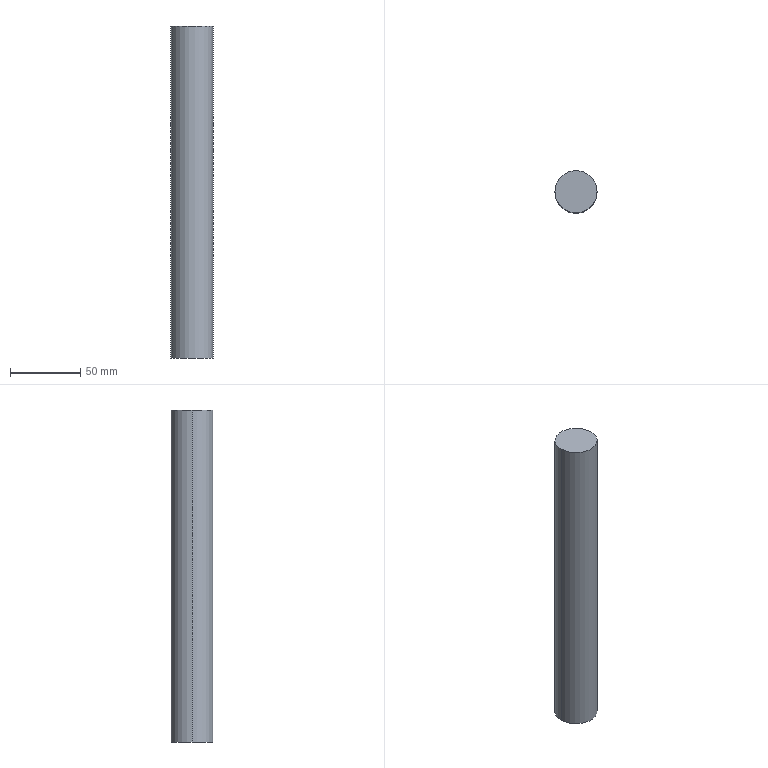Part | SolidWorks | features Extrusion 1 | 1 solid | 4 faces | box 30 x 30 x 236 mm | volume 166819 mm3 | cylinder 2 | plane 2 | commonest cylinder face diameters 30 x2
STEP:
#1=CARTESIAN_POINT('',(15.,0.,236.));
#2=VERTEX_POINT('',#1);
#3=CARTESIAN_POINT('',(-15.,0.,236.));
#4=VERTEX_POINT('',#3);
#5=CARTESIAN_POINT('',(0.,0.,236.));
#6=DIRECTION('',(0.,0.,1.));
#7=DIRECTION('',(1.,0.,0.));
#8=AXIS2_PLACEMENT_3D('',#5,#6,#7);
#9=CIRCLE('',#8,15.);
#10=EDGE_CURVE('',#2,#4,#9,.T.);
#11=ORIENTED_EDGE('',*,*,#10,.F.);
#12=CARTESIAN_POINT('',(15.,0.,0.));
#13=VERTEX_POINT('',#12);
#14=CARTESIAN_POINT('',(15.,0.,236.));
#15=DIRECTION('',(0.,0.,-1.));
#16=VECTOR('',#15,1000.);
#17=LINE('',#14,#16);
#18=EDGE_CURVE('',#2,#13,#17,.T.);
#19=ORIENTED_EDGE('',*,*,#18,.T.);
#20=CARTESIAN_POINT('',(-15.,0.,0.));
#21=VERTEX_POINT('',#20);
#22=CARTESIAN_POINT('',(0.,0.,0.));
#23=DIRECTION('',(0.,0.,1.));
#24=DIRECTION('',(1.,0.,0.));
#25=AXIS2_PLACEMENT_3D('',#22,#23,#24);
#26=CIRCLE('',#25,15.);
#27=EDGE_CURVE('',#13,#21,#26,.T.);
#28=ORIENTED_EDGE('',*,*,#27,.T.);
#29=CARTESIAN_POINT('',(-15.,0.,236.));
#30=DIRECTION('',(0.,0.,-1.));
#31=VECTOR('',#30,1000.);
#32=LINE('',#29,#31);
#33=EDGE_CURVE('',#4,#21,#32,.T.);
#34=ORIENTED_EDGE('',*,*,#33,.F.);
#35=EDGE_LOOP('',(#11,#19,#28,#34));
#36=FACE_OUTER_BOUND('',#35,.T.);
#37=CARTESIAN_POINT('',(0.,0.,236.));
#38=DIRECTION('',(0.,0.,-1.));
#39=DIRECTION('',(-1.,0.,0.));
#40=AXIS2_PLACEMENT_3D('',#37,#38,#39);
#41=CYLINDRICAL_SURFACE('',#40,15.);
#42=ADVANCED_FACE('',(#36),#41,.T.);
#43=ORIENTED_EDGE('',*,*,#18,.F.);
#44=CARTESIAN_POINT('',(0.,0.,236.));
#45=DIRECTION('',(0.,0.,1.));
#46=DIRECTION('',(1.,0.,0.));
#47=AXIS2_PLACEMENT_3D('',#44,#45,#46);
#48=CIRCLE('',#47,15.);
#49=EDGE_CURVE('',#4,#2,#48,.T.);
#50=ORIENTED_EDGE('',*,*,#49,.F.);
#51=ORIENTED_EDGE('',*,*,#33,.T.);
#52=CARTESIAN_POINT('',(0.,0.,0.));
#53=DIRECTION('',(0.,0.,1.));
#54=DIRECTION('',(1.,0.,0.));
#55=AXIS2_PLACEMENT_3D('',#52,#53,#54);
#56=CIRCLE('',#55,15.);
#57=EDGE_CURVE('',#21,#13,#56,.T.);
#58=ORIENTED_EDGE('',*,*,#57,.T.);
#59=EDGE_LOOP('',(#43,#50,#51,#58));
#60=FACE_OUTER_BOUND('',#59,.T.);
#61=CARTESIAN_POINT('',(0.,0.,236.));
#62=DIRECTION('',(0.,0.,-1.));
#63=DIRECTION('',(-1.,0.,0.));
#64=AXIS2_PLACEMENT_3D('',#61,#62,#63);
#65=CYLINDRICAL_SURFACE('',#64,15.);
#66=ADVANCED_FACE('',(#60),#65,.T.);
#67=ORIENTED_EDGE('',*,*,#49,.T.);
#68=ORIENTED_EDGE('',*,*,#10,.T.);
#69=EDGE_LOOP('',(#67,#68));
#70=FACE_OUTER_BOUND('',#69,.T.);
#71=CARTESIAN_POINT('',(0.,0.,236.));
#72=DIRECTION('',(0.,0.,1.));
#73=DIRECTION('',(1.,0.,0.));
#74=AXIS2_PLACEMENT_3D('',#71,#72,#73);
#75=PLANE('',#74);
#76=ADVANCED_FACE('',(#70),#75,.T.);
#77=ORIENTED_EDGE('',*,*,#57,.F.);
#78=ORIENTED_EDGE('',*,*,#27,.F.);
#79=EDGE_LOOP('',(#77,#78));
#80=FACE_OUTER_BOUND('',#79,.T.);
#81=CARTESIAN_POINT('',(0.,0.,0.));
#82=DIRECTION('',(0.,0.,1.));
#83=DIRECTION('',(1.,0.,0.));
#84=AXIS2_PLACEMENT_3D('',#81,#82,#83);
#85=PLANE('',#84);
#86=ADVANCED_FACE('',(#80),#85,.F.);
#87=CLOSED_SHELL('',(#42,#66,#76,#86));
#88=MANIFOLD_SOLID_BREP('',#87);
#89=CARTESIAN_POINT('',(0.,0.,0.));
#90=DIRECTION('',(0.,0.,1.));
#91=DIRECTION('',(1.,0.,0.));
#92=AXIS2_PLACEMENT_3D('',#89,#90,#91);
#93=(LENGTH_UNIT()NAMED_UNIT(*)SI_UNIT(.MILLI.,.METRE.));
#94=UNCERTAINTY_MEASURE_WITH_UNIT(LENGTH_MEASURE(0.00001),#93,'','');
#95=(NAMED_UNIT(*)PLANE_ANGLE_UNIT()SI_UNIT($,.RADIAN.));
#96=(NAMED_UNIT(*)SI_UNIT($,.STERADIAN.)SOLID_ANGLE_UNIT());
#97=(GEOMETRIC_REPRESENTATION_CONTEXT(3)GLOBAL_UNCERTAINTY_ASSIGNED_CONTEXT((#94))GLOBAL_UNIT_ASSIGNED_CONTEXT((#93,#95,#96))REPRESENTATION_CONTEXT('',''));
#98=ADVANCED_BREP_SHAPE_REPRESENTATION('',(#88,#92),#97);